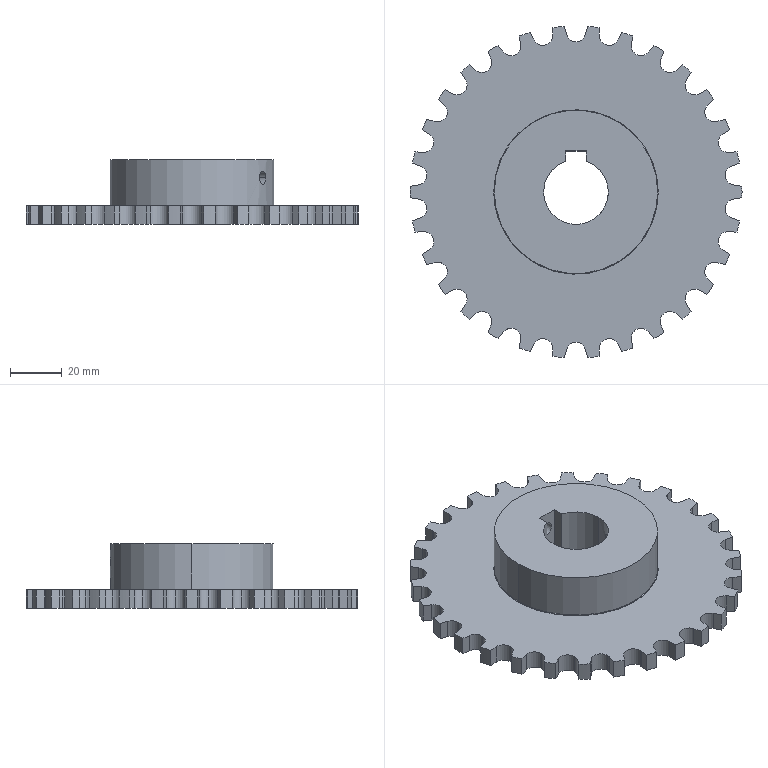Part | STEP file | 1004-2001-0088_1004-2001-0088_1-2 | 1 solid | 150 faces | box 128 x 127.688 x 25 mm | volume 125433 mm3 | cylinder 82 | plane 66 | spline 2 | commonest cylinder face diameters 7.5 x42 128 x31 5 x4 25 x3 63 x2